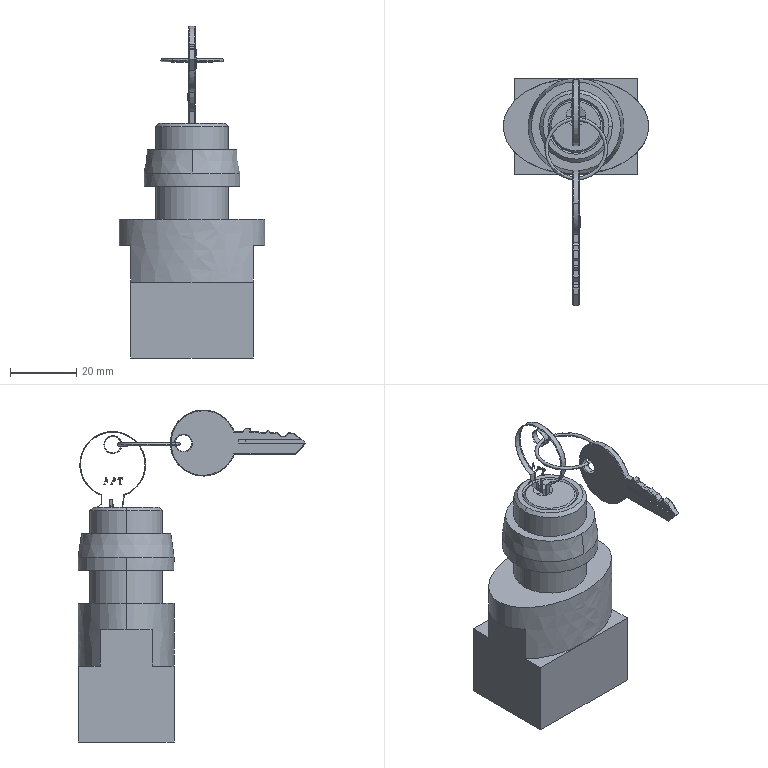Part | NX | features BREP 8 | 2 solids | 229 faces | box 44 x 68.858 x 100.5 mm | volume 36069 mm3 | plane 156 | spline 28 | cone 27 | cylinder 14 | torus 4 | commonest cylinder face diameters 5 x4 20 x4 22 x4 29 x2